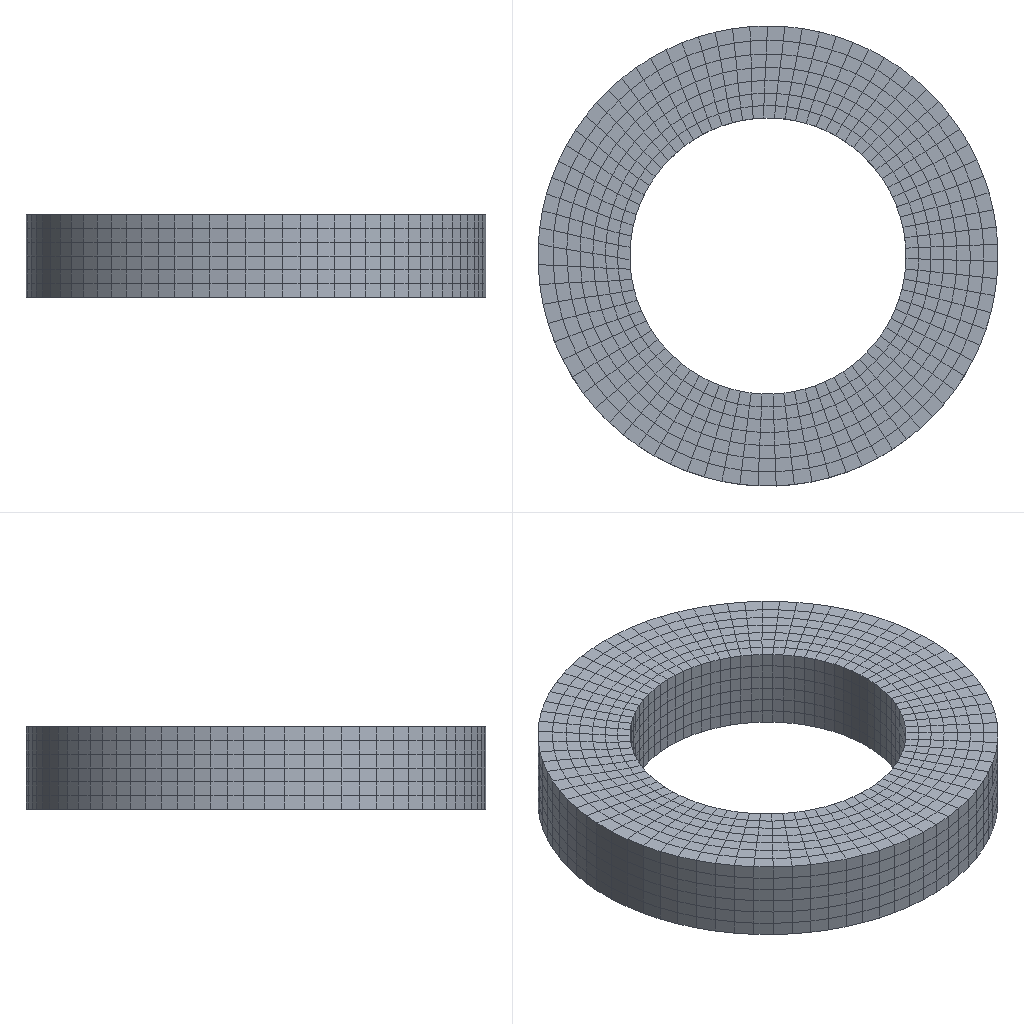Simulation study | abaqus
Set-up summary:
category,name,step,type,value,unit,region
solver,abaqus
solver,version,,,Abaqus/Standard 2020
units,not stated in the deck,,not stated
analysis,deck,,transient,transient
load_step,Step-1,Step-1,transient,nlgeom=True
load_step,Step-2,Step-2,transient,nlgeom=True
contact,interactions,,,general=0 pairs=1 ties=0
load_step,requested,,,2
mesh,nodes,,,5578
mesh,elements,,,4440
element_type,R3D4,,rigid,1038
element_type,C3D8RH,,solid,3402
load,load commands in deck,,count,3
bc,support commands in deck,,count,23
material,PU,,in results
check,setup vs results,,match,"per instance, exact: element labels, types and connectivity; labels of the nodes the elements use; coordinates of those nodes at SINGLE_PRECISION in 2 of 2 instance(s)"
Abaqus input file, long lists of numbers shortened, first 1954 of 6997 lines:
*Heading
** Job name: Job-1 Model name: Job-stress
** Generated by: Abaqus/CAE 2020
*Preprint, echo=NO, model=NO, history=NO, contact=NO
**
** PARTS
**
*Part, name=PART-1
*Node
      1,   21.965,   44.917,           0.
      2,   12.595,   27.228,           0.
** (4535 more lines like these left out)
*Element, type=C3D8RH
   1,  649,  659,  841,  720,    1,   11,  193,   72
   2,  659,  660,  842,  841,   11,   12,  194,  193
** (3400 more lines like these left out)
*Elset, elset=PART-1-1_SHIXINTAI, generate
    1,  3402,     1
** Section: Section-1-PART-1-1_SHIXINTAI
*Solid Section, elset=PART-1-1_SHIXINTAI, material=PU
,
*End Part
**
*Part, name=road
*Node
      1,         200.,           0.,           1.
      2,         200.,        -150.,           1.
** (1038 more lines like these left out)
*Element, type=R3D4
 1,  1,  9, 44,  4
 2,  9, 10, 43, 44
** (1036 more lines like these left out)
*Node
   1041,         100.,         -75.,           0.
*Nset, nset=road-RefPt_, internal
1041,
*Elset, elset=road, generate
    1,  1038,     1
*End Part
**
**
** ASSEMBLY
**
*Assembly, name=Assembly
**
*Instance, name=PART-1-1, part=PART-1
*End Instance
**
*Instance, name=road-1, part=road
         20.,         -51.,         -85.
         20.,         -51.,         -85.,          20., -50.293, -85.707,         180.
*End Instance
**
*Nset, nset=PART-1-1_NEI-RP, instance=PART-1-1
 4537,
*Nset, nset=Set-3417, instance=road-1
 1041,
*Nset, nset=PART-1-1-REFPT_, internal, instance=PART-1-1
 4537,
*Elset, elset=_M18, internal, instance=PART-1-1
 1188,
*Elset, elset=_M19, internal, instance=PART-1-1
 1181,
*Elset, elset=_M20, internal, instance=PART-1-1
 1755,
*Elset, elset=_M21, internal, instance=PART-1-1
 1174,
*Elset, elset=_M22, internal, instance=PART-1-1
 1087,
*Elset, elset=_M23, internal, instance=PART-1-1
 1655,
*Elset, elset=_M24, internal, instance=PART-1-1
 1195,
*Elset, elset=_M25, internal, instance=PART-1-1
 1648,
*Elset, elset=_M26, internal, instance=PART-1-1
 1762,
*Elset, elset=_M27, internal, instance=PART-1-1
 1748,
*Elset, elset=_M28, internal, instance=PART-1-1
 1634,
*Elset, elset=_M29, internal, instance=PART-1-1
 1641,
*Elset, elset=_M30, internal, instance=PART-1-1
 1167,
*Elset, elset=_M31, internal, instance=PART-1-1
 1662,
*Elset, elset=_M32, internal, instance=PART-1-1
 1202,
*Elset, elset=_M33, internal, instance=PART-1-1
 1769,
*Elset, elset=_M34, internal, instance=PART-1-1
 2229,
*Elset, elset=_M35, internal, instance=PART-1-1
 1073,
*Elset, elset=_M36, internal, instance=PART-1-1
 1091,
*Elset, elset=_M37, internal, instance=PART-1-1
 1180,
*Elset, elset=_M38, internal, instance=PART-1-1
 1741,
*Elset, elset=_M39, internal, instance=PART-1-1
 1084,
*Elset, elset=_M40, internal, instance=PART-1-1
 2215,
*Elset, elset=_M41, internal, instance=PART-1-1
 1187,
*Elset, elset=_M42, internal, instance=PART-1-1
 1063,
*Elset, elset=_M43, internal, instance=PART-1-1
 1642,
*Elset, elset=_M44, internal, instance=PART-1-1
 1650,
*Elset, elset=_M45, internal, instance=PART-1-1
 1098,
*Elset, elset=_M46, internal, instance=PART-1-1
 1194,
*Elset, elset=_M47, internal, instance=PART-1-1
 1649,
*Elset, elset=_M48, internal, instance=PART-1-1
 1172,
*Elset, elset=_M49, internal, instance=PART-1-1
 1656,
*Elset, elset=_M50, internal, instance=PART-1-1
 1643,
*Elset, elset=_M51, internal, instance=PART-1-1
 1179,
*Elset, elset=_M52, internal, instance=PART-1-1
 1166,
*Elset, elset=_M53, internal, instance=PART-1-1
 2236,
*Elset, elset=_M54, internal, instance=PART-1-1
 1173,
*Elset, elset=_M55, internal, instance=PART-1-1
 1663,
*Elset, elset=_M56, internal, instance=PART-1-1
 1669,
*Elset, elset=_M57, internal, instance=PART-1-1
 1627,
*Elset, elset=_M58, internal, instance=PART-1-1
 2208,
*Elset, elset=_M59, internal, instance=PART-1-1
 1160,
*Elset, elset=_M60, internal, instance=PART-1-1
 1165,
*Elset, elset=_M61, internal, instance=PART-1-1
 1761,
*Elset, elset=_M62, internal, instance=PART-1-1
 1635,
*Elset, elset=_M63, internal, instance=PART-1-1
 2222,
*Elset, elset=_M64, internal, instance=PART-1-1
 1754,
*Elset, elset=_M65, internal, instance=PART-1-1
 1657,
*Elset, elset=_M66, internal, instance=PART-1-1
 1636,
*Elset, elset=_M67, internal, instance=PART-1-1
 2217,
*Elset, elset=_M68, internal, instance=PART-1-1
 1159,
*Elset, elset=_M69, internal, instance=PART-1-1
 1201,
*Elset, elset=_M70, internal, instance=PART-1-1
 1768,
*Elset, elset=_M71, internal, instance=PART-1-1
 1059,
*Elset, elset=_M72, internal, instance=PART-1-1
 1209,
*Elset, elset=_M73, internal, instance=PART-1-1
 1186,
*Elset, elset=_M74, internal, instance=PART-1-1
 1747,
*Elset, elset=_M75, internal, instance=PART-1-1
 1776,
*Elset, elset=_M76, internal, instance=PART-1-1
 2194,
*Elset, elset=_M77, internal, instance=PART-1-1
 1734,
*Elset, elset=_M78, internal, instance=PART-1-1
 2788,
*Elset, elset=_M79, internal, instance=PART-1-1
 2210,
*Elset, elset=_M80, internal, instance=PART-1-1
 601,
*Elset, elset=_M81, internal, instance=PART-1-1
 611,
*Elset, elset=_M82, internal, instance=PART-1-1
 1629,
*Elset, elset=_M83, internal, instance=PART-1-1
 2201,
*Elset, elset=_M84, internal, instance=PART-1-1
 2230,
*Elset, elset=_M85, internal, instance=PART-1-1
 1670,
*Elset, elset=_M86, internal, instance=PART-1-1
 1628,
*Elset, elset=_M87, internal, instance=PART-1-1
 1753,
*Elset, elset=_M88, internal, instance=PART-1-1
 2223,
*Elset, elset=_M89, internal, instance=PART-1-1
 1746,
*Elset, elset=_M90, internal, instance=PART-1-1
 2209,
*Elset, elset=_M91, internal, instance=PART-1-1
 1193,
*Elset, elset=_M92, internal, instance=PART-1-1
 1739,
*Elset, elset=_M93, internal, instance=PART-1-1
 1153,
*Elset, elset=_M94, internal, instance=PART-1-1
 1740,
*Elset, elset=_M95, internal, instance=PART-1-1
 2216,
*Elset, elset=_M96, internal, instance=PART-1-1
 2224,
*Elset, elset=_M97, internal, instance=PART-1-1
 1676,
*Elset, elset=_M98, internal, instance=PART-1-1
 594,
*Elset, elset=_M99, internal, instance=PART-1-1
 1760,
*Elset, elset=_M100, internal, instance=PART-1-1
 1208,
*Elset, elset=_M101, internal, instance=PART-1-1
 1158,
*Elset, elset=_M102, internal, instance=PART-1-1
 597,
*Elset, elset=_M103, internal, instance=PART-1-1
 1664,
*Elset, elset=_M104, internal, instance=PART-1-1
 2237,
*Elset, elset=_M105, internal, instance=PART-1-1
 1066,
*Elset, elset=_M106, internal, instance=PART-1-1
 1200,
*Elset, elset=_M107, internal, instance=PART-1-1
 1775,
*Elset, elset=_M108, internal, instance=PART-1-1
 1733,
*Elset, elset=_M109, internal, instance=PART-1-1
 1620,
*Elset, elset=_M110, internal, instance=PART-1-1
 1767,
*Elset, elset=_M111, internal, instance=PART-1-1
 1732,
*Elset, elset=_M112, internal, instance=PART-1-1
 2243,
*Elset, elset=_M113, internal, instance=PART-1-1
 1677,
*Elset, elset=_M114, internal, instance=PART-1-1
 1727,
*Elset, elset=_M115, internal, instance=PART-1-1
 1152,
*Elset, elset=_M116, internal, instance=PART-1-1
 1725,
*Elset, elset=_M117, internal, instance=PART-1-1
 604,
*Elset, elset=_M118, internal, instance=PART-1-1
 1726,
*Elset, elset=_M119, internal, instance=PART-1-1
 1621,
*Elset, elset=_M120, internal, instance=PART-1-1
 1749,
*Elset, elset=_M121, internal, instance=PART-1-1
 2203,
*Elset, elset=_M122, internal, instance=PART-1-1
 1207,
*Elset, elset=_M123, internal, instance=PART-1-1
 1182,
*Elset, elset=_M124, internal, instance=PART-1-1
 1720,
*Elset, elset=_M125, internal, instance=PART-1-1
 590,
*Elset, elset=_M126, internal, instance=PART-1-1
 1151,
*Elset, elset=_M127, internal, instance=PART-1-1
 1489,
*Elset, elset=_M128, internal, instance=PART-1-1
 615,
*Elset, elset=_M129, internal, instance=PART-1-1
 1719,
*Elset, elset=_M130, internal, instance=PART-1-1
 2231,
*Elset, elset=_M131, internal, instance=PART-1-1
 1622,
*Elset, elset=_M132, internal, instance=PART-1-1
 1671,
*Elset, elset=_M133, internal, instance=PART-1-1
 1215,
*Elset, elset=_M134, internal, instance=PART-1-1
 2244,
*Elset, elset=_M135, internal, instance=PART-1-1
 2187,
*Elset, elset=_M136, internal, instance=PART-1-1
 2202,
*Elset, elset=_M137, internal, instance=PART-1-1
 1774,
*Elset, elset=_M138, internal, instance=PART-1-1
 1145,
*Elset, elset=_M139, internal, instance=PART-1-1
 1496,
*Elset, elset=_M140, internal, instance=PART-1-1
 1488,
*Elset, elset=_M141, internal, instance=PART-1-1
 1216,
*Elset, elset=_M142, internal, instance=PART-1-1
 608,
*Elset, elset=_M143, internal, instance=PART-1-1
 622,
*Elset, elset=_M144, internal, instance=PART-1-1
 2056,
*Elset, elset=_M145, internal, instance=PART-1-1
 1146,
*Elset, elset=_M146, internal, instance=PART-1-1
 2340,
*Elset, elset=_M147, internal, instance=PART-1-1
 1782,
*Elset, elset=_M148, internal, instance=PART-1-1
 1712,
*Elset, elset=_M149, internal, instance=PART-1-1
 2063,
*Elset, elset=_M150, internal, instance=PART-1-1
 1077,
*Elset, elset=_M151, internal, instance=PART-1-1
 1214,
*Elset, elset=_M152, internal, instance=PART-1-1
 1713,
*Elset, elset=_M153, internal, instance=PART-1-1
 2189,
*Elset, elset=_M154, internal, instance=PART-1-1
 1718,
*Elset, elset=_M155, internal, instance=PART-1-1
 919,
*Elset, elset=_M156, internal, instance=PART-1-1
 2238,
*Elset, elset=_M157, internal, instance=PART-1-1
 1783,
*Elset, elset=_M158, internal, instance=PART-1-1
 2055,
*Elset, elset=_M159, internal, instance=PART-1-1
 2207,
*Elset, elset=_M160, internal, instance=PART-1-1
 2195,
*Elset, elset=_M161, internal, instance=PART-1-1
 1495,
*Elset, elset=_M162, internal, instance=PART-1-1
 1684,
*Elset, elset=_M163, internal, instance=PART-1-1
 2196,
*Elset, elset=_M164, internal, instance=PART-1-1
 1503,
*Elset, elset=_M165, internal, instance=PART-1-1
 1711,
*Elset, elset=_M166, internal, instance=PART-1-1
 1144,
*Elset, elset=_M167, internal, instance=PART-1-1
 1138,
*Elset, elset=_M168, internal, instance=PART-1-1
 2070,
*Elset, elset=_M169, internal, instance=PART-1-1
 2188,
*Elset, elset=_M170, internal, instance=PART-1-1
 1678,
*Elset, elset=_M171, internal, instance=PART-1-1
 2062,
*Elset, elset=_M172, internal, instance=PART-1-1
 1487,
*Elset, elset=_M173, internal, instance=PART-1-1
 2245,
*Elset, elset=_M174, internal, instance=PART-1-1
 2799,
*Elset, elset=_M175, internal, instance=PART-1-1
 1683,
*Elset, elset=_M176, internal, instance=PART-1-1
 1222,
*Elset, elset=_M177, internal, instance=PART-1-1
 1139,
*Elset, elset=_M178, internal, instance=PART-1-1
 1781,
*Elset, elset=_M179, internal, instance=PART-1-1
 1055,
*Elset, elset=_M180, internal, instance=PART-1-1
 1705,
*Elset, elset=_M181, internal, instance=PART-1-1
 629,
*Elset, elset=_M182, internal, instance=PART-1-1
 2250,
*Elset, elset=_M183, internal, instance=PART-1-1
 1223,
*Elset, elset=_M184, internal, instance=PART-1-1
 1706,
*Elset, elset=_M185, internal, instance=PART-1-1
 1790,
*Elset, elset=_M186, internal, instance=PART-1-1
 1789,
*Elset, elset=_M187, internal, instance=PART-1-1
 1137,
*Elset, elset=_M188, internal, instance=PART-1-1
 1052,
*Elset, elset=_M189, internal, instance=PART-1-1
 1502,
*Elset, elset=_M190, internal, instance=PART-1-1
 1704,
*Elset, elset=_M191, internal, instance=PART-1-1
 2251,
*Elset, elset=_M192, internal, instance=PART-1-1
 2312,
*Elset, elset=_M193, internal, instance=PART-1-1
 587,
*Elset, elset=_M194, internal, instance=PART-1-1
 2069,
*Elset, elset=_M195, internal, instance=PART-1-1
 2809,
*Elset, elset=_M196, internal, instance=PART-1-1
 2291,
*Elset, elset=_M197, internal, instance=PART-1-1
 1685,
*Elset, elset=_M198, internal, instance=PART-1-1
 2802,
*Elset, elset=_M199, internal, instance=PART-1-1
 2760,
*Elset, elset=_M200, internal, instance=PART-1-1
 1101,
*Elset, elset=_M201, internal, instance=PART-1-1
 2781,
*Elset, elset=_M202, internal, instance=PART-1-1
 1320,
*Elset, elset=_M203, internal, instance=PART-1-1
 2252,
*Elset, elset=_M204, internal, instance=PART-1-1
 1509,
*Elset, elset=_M205, internal, instance=PART-1-1
 2054,
*Elset, elset=_M206, internal, instance=PART-1-1
 2077,
*Elset, elset=_M207, internal, instance=PART-1-1
 1221,
*Elset, elset=_M208, internal, instance=PART-1-1
 1229,
*Elset, elset=_M209, internal, instance=PART-1-1
 1494,
*Elset, elset=_M210, internal, instance=PART-1-1
 1886,
*Elset, elset=_M211, internal, instance=PART-1-1
 1691,
*Elset, elset=_M212, internal, instance=PART-1-1
 2753,
*Elset, elset=_M213, internal, instance=PART-1-1
 1887,
*Elset, elset=_M214, internal, instance=PART-1-1
 1510,
*Elset, elset=_M215, internal, instance=PART-1-1
 1319,
*Elset, elset=_M216, internal, instance=PART-1-1
 1230,
*Elset, elset=_M217, internal, instance=PART-1-1
 583,
*Elset, elset=_M218, internal, instance=PART-1-1
 947,
*Elset, elset=_M219, internal, instance=PART-1-1
 1796,
*Elset, elset=_M220, internal, instance=PART-1-1
 1788,
*Elset, elset=_M221, internal, instance=PART-1-1
 2061,
*Elset, elset=_M222, internal, instance=PART-1-1
 1797,
*Elset, elset=_M223, internal, instance=PART-1-1
 1074,
*Elset, elset=_M224, internal, instance=PART-1-1
 2813,
*Elset, elset=_M225, internal, instance=PART-1-1
 2309,
*Elset, elset=_M226, internal, instance=PART-1-1
 1501,
*Elset, elset=_M227, internal, instance=PART-1-1
 2076,
*Elset, elset=_M228, internal, instance=PART-1-1
 2774,
*Elset, elset=_M229, internal, instance=PART-1-1
 2638,
*Elset, elset=_M230, internal, instance=PART-1-1
 755,
*Elset, elset=_M231, internal, instance=PART-1-1
 2277,
*Elset, elset=_M232, internal, instance=PART-1-1
 1516,
*Elset, elset=_M233, internal, instance=PART-1-1
 1893,
*Elset, elset=_M234, internal, instance=PART-1-1
 2764,
*Elset, elset=_M235, internal, instance=PART-1-1
 1321,
*Elset, elset=_M236, internal, instance=PART-1-1
 1692,
*Elset, elset=_M237, internal, instance=PART-1-1
 2075,
*Elset, elset=_M238, internal, instance=PART-1-1
 1508,
*Elset, elset=_M239, internal, instance=PART-1-1
 1185,
*Elset, elset=_M240, internal, instance=PART-1-1
 1894,
*Elset, elset=_M241, internal, instance=PART-1-1
 1327,
*Elset, elset=_M242, internal, instance=PART-1-1
 1690,
*Elset, elset=_M243, internal, instance=PART-1-1
 2084,
*Elset, elset=_M244, internal, instance=PART-1-1
 1326,
*Elset, elset=_M245, internal, instance=PART-1-1
 1888,
*Elset, elset=_M246, internal, instance=PART-1-1
 2068,
*Elset, elset=_M247, internal, instance=PART-1-1
 1517,
*Elset, elset=_M248, internal, instance=PART-1-1
 2258,
*Elset, elset=_M249, internal, instance=PART-1-1
 2083,
*Elset, elset=_M250, internal, instance=PART-1-1
 2757,
*Elset, elset=_M251, internal, instance=PART-1-1
 2284,
*Elset, elset=_M252, internal, instance=PART-1-1
 2270,
*Elset, elset=_M253, internal, instance=PART-1-1
 1126,
*Elset, elset=_M254, internal, instance=PART-1-1
 2771,
*Elset, elset=_M255, internal, instance=PART-1-1
 1228,
*Elset, elset=_M256, internal, instance=PART-1-1
 2778,
*Elset, elset=_M257, internal, instance=PART-1-1
 1164,
*Elset, elset=_M258, internal, instance=PART-1-1
 1236,
*Elset, elset=_M259, internal, instance=PART-1-1
 1088,
*Elset, elset=_M260, internal, instance=PART-1-1
 2305,
*Elset, elset=_M261, internal, instance=PART-1-1
 2624,
*Elset, elset=_M262, internal, instance=PART-1-1
 1334,
*Elset, elset=_M263, internal, instance=PART-1-1
 2257,
*Elset, elset=_M264, internal, instance=PART-1-1
 1119,
*Elset, elset=_M265, internal, instance=PART-1-1
 2259,
*Elset, elset=_M266, internal, instance=PART-1-1
 1803,
*Elset, elset=_M267, internal, instance=PART-1-1
 1515,
*Elset, elset=_M268, internal, instance=PART-1-1
 1901,
*Elset, elset=_M269, internal, instance=PART-1-1
 2456,
*Elset, elset=_M270, internal, instance=PART-1-1
 1698,
*Elset, elset=_M271, internal, instance=PART-1-1
 1640,
*Elset, elset=_M272, internal, instance=PART-1-1
 1333,
*Elset, elset=_M273, internal, instance=PART-1-1
 643,
*Elset, elset=_M274, internal, instance=PART-1-1
 569,
*Elset, elset=_M275, internal, instance=PART-1-1
 1237,
*Elset, elset=_M276, internal, instance=PART-1-1
 2057,
*Elset, elset=_M277, internal, instance=PART-1-1
 2326,
*Elset, elset=_M278, internal, instance=PART-1-1
 765,
*Elset, elset=_M279, internal, instance=PART-1-1
 1795,
*Elset, elset=_M280, internal, instance=PART-1-1
 1112,
*Elset, elset=_M281, internal, instance=PART-1-1
 1900,
*Elset, elset=_M282, internal, instance=PART-1-1
 626,
*Elset, elset=_M283, internal, instance=PART-1-1
 1523,
*Elset, elset=_M284, internal, instance=PART-1-1
 2082,
*Elset, elset=_M285, internal, instance=PART-1-1
 1895,
*Elset, elset=_M286, internal, instance=PART-1-1
 1752,
*Elset, elset=_M287, internal, instance=PART-1-1
 2298,
*Elset, elset=_M288, internal, instance=PART-1-1
 1341,
*Elset, elset=_M289, internal, instance=PART-1-1
 2090,
*Elset, elset=_M290, internal, instance=PART-1-1
 636,
*Elset, elset=_M291, internal, instance=PART-1-1
 607,
*Elset, elset=_M292, internal, instance=PART-1-1
 1908,
*Elset, elset=_M293, internal, instance=PART-1-1
 1056,
*Elset, elset=_M294, internal, instance=PART-1-1
 758,
*Elset, elset=_M295, internal, instance=PART-1-1
 2816,
*Elset, elset=_M296, internal, instance=PART-1-1
 1637,
*Elset, elset=_M297, internal, instance=PART-1-1
 2823,
*Elset, elset=_M298, internal, instance=PART-1-1
 1243,
*Elset, elset=_M299, internal, instance=PART-1-1
 1328,
*Elset, elset=_M300, internal, instance=PART-1-1
 1804,
*Elset, elset=_M301, internal, instance=PART-1-1
 2767,
*Elset, elset=_M302, internal, instance=PART-1-1
 1697,
*Elset, elset=_M303, internal, instance=PART-1-1
 2089,
*Elset, elset=_M304, internal, instance=PART-1-1
 1340,
*Elset, elset=_M305, internal, instance=PART-1-1
 1171,
*Elset, elset=_M306, internal, instance=PART-1-1
 2091,
*Elset, elset=_M307, internal, instance=PART-1-1
 1129,
*Elset, elset=_M308, internal, instance=PART-1-1
 2795,
*Elset, elset=_M309, internal, instance=PART-1-1
 580,
*Elset, elset=_M310, internal, instance=PART-1-1
 1522,
*Elset, elset=_M311, internal, instance=PART-1-1
 1335,
*Elset, elset=_M312, internal, instance=PART-1-1
 1524,
*Elset, elset=_M313, internal, instance=PART-1-1
 1907,
*Elset, elset=_M314, internal, instance=PART-1-1
 2265,
*Elset, elset=_M315, internal, instance=PART-1-1
 1235,
*Elset, elset=_M316, internal, instance=PART-1-1
 2652,
*Elset, elset=_M317, internal, instance=PART-1-1
 1699,
*Elset, elset=_M318, internal, instance=PART-1-1
 975,
*Elset, elset=_M319, internal, instance=PART-1-1
 1902,
*Elset, elset=_M320, internal, instance=PART-1-1
 2645,
*Elset, elset=_M321, internal, instance=PART-1-1
 618,
*Elset, elset=_M322, internal, instance=PART-1-1
 1530,
*Elset, elset=_M323, internal, instance=PART-1-1
 1411,
*Elset, elset=_M324, internal, instance=PART-1-1
 1213,
*Elset, elset=_M325, internal, instance=PART-1-1
 2264,
*Elset, elset=_M326, internal, instance=PART-1-1
 642,
*Elset, elset=_M327, internal, instance=PART-1-1
 1802,
*Elset, elset=_M328, internal, instance=PART-1-1
 2329,
*Elset, elset=_M329, internal, instance=PART-1-1
 1490,
*Elset, elset=_M330, internal, instance=PART-1-1
 632,
*Elset, elset=_M331, internal, instance=PART-1-1
 1892,
*Elset, elset=_M332, internal, instance=PART-1-1
 2477,
*Elset, elset=_M333, internal, instance=PART-1-1
 922,
*Elset, elset=_M334, internal, instance=PART-1-1
 1810,
*Elset, elset=_M335, internal, instance=PART-1-1
 958,
*Elset, elset=_M336, internal, instance=PART-1-1
 1348,
*Elset, elset=_M337, internal, instance=PART-1-1
 2266,
*Elset, elset=_M338, internal, instance=PART-1-1
 776,
*Elset, elset=_M339, internal, instance=PART-1-1
 1242,
*Elset, elset=_M340, internal, instance=PART-1-1
 2323,
*Elset, elset=_M341, internal, instance=PART-1-1
 2335,
*Elset, elset=_M342, internal, instance=PART-1-1
 2806,
*Elset, elset=_M343, internal, instance=PART-1-1
 1250,
*Elset, elset=_M344, internal, instance=PART-1-1
 1909,
*Elset, elset=_M345, internal, instance=PART-1-1
 1889,
*Elset, elset=_M346, internal, instance=PART-1-1
 1915,
*Elset, elset=_M347, internal, instance=PART-1-1
 2470,
*Elset, elset=_M348, internal, instance=PART-1-1
 1342,
*Elset, elset=_M349, internal, instance=PART-1-1
 951,
*Elset, elset=_M350, internal, instance=PART-1-1
 2097,
*Elset, elset=_M351, internal, instance=PART-1-1
 598,
*Elset, elset=_M352, internal, instance=PART-1-1
 2281,
*Elset, elset=_M353, internal, instance=PART-1-1
 2344,
*Elset, elset=_M354, internal, instance=PART-1-1
 1102,
*Elset, elset=_M355, internal, instance=PART-1-1
 1244,
*Elset, elset=_M356, internal, instance=PART-1-1
 1097,
*Elset, elset=_M357, internal, instance=PART-1-1
 1809,
*Elset, elset=_M358, internal, instance=PART-1-1
 619,
*Elset, elset=_M359, internal, instance=PART-1-1
 579,
*Elset, elset=_M360, internal, instance=PART-1-1
 1322,
*Elset, elset=_M361, internal, instance=PART-1-1
 1110,
*Elset, elset=_M362, internal, instance=PART-1-1
 1412,
*Elset, elset=_M363, internal, instance=PART-1-1
 1531,
*Elset, elset=_M364, internal, instance=PART-1-1
 1410,
*Elset, elset=_M365, internal, instance=PART-1-1
 2827,
*Elset, elset=_M366, internal, instance=PART-1-1
 592,
*Elset, elset=_M367, internal, instance=PART-1-1
 1529,
*Elset, elset=_M368, internal, instance=PART-1-1
 2820,
*Elset, elset=_M369, internal, instance=PART-1-1
 2634,
*Elset, elset=_M370, internal, instance=PART-1-1
 2186,
*Elset, elset=_M371, internal, instance=PART-1-1
 1537,
*Elset, elset=_M372, internal, instance=PART-1-1
 1978,
*Elset, elset=_M373, internal, instance=PART-1-1
 1977,
*Elset, elset=_M374, internal, instance=PART-1-1
 1916,
*Elset, elset=_M375, internal, instance=PART-1-1
 2096,
*Elset, elset=_M376, internal, instance=PART-1-1
 2204,
*Elset, elset=_M377, internal, instance=PART-1-1
 1083,
*Elset, elset=_M378, internal, instance=PART-1-1
 2358,
*Elset, elset=_M379, internal, instance=PART-1-1
 1061,
*Elset, elset=_M380, internal, instance=PART-1-1
 1178,
*Elset, elset=_M381, internal, instance=PART-1-1
 2659,
*Elset, elset=_M382, internal, instance=PART-1-1
 769,
*Elset, elset=_M383, internal, instance=PART-1-1
 1418,
*Elset, elset=_M384, internal, instance=PART-1-1
 1355,
*Elset, elset=_M385, internal, instance=PART-1-1
 2098,
*Elset, elset=_M386, internal, instance=PART-1-1
 1672,
*Elset, elset=_M387, internal, instance=PART-1-1
 640,
*Elset, elset=_M388, internal, instance=PART-1-1
 2239,
*Elset, elset=_M389, internal, instance=PART-1-1
 1914,
*Elset, elset=_M390, internal, instance=PART-1-1
 1922,
*Elset, elset=_M391, internal, instance=PART-1-1
 2830,
*Elset, elset=_M392, internal, instance=PART-1-1
 1349,
*Elset, elset=_M393, internal, instance=PART-1-1
 944,
*Elset, elset=_M394, internal, instance=PART-1-1
 2459,
*Elset, elset=_M395, internal, instance=PART-1-1
 2306,
*Elset, elset=_M396, internal, instance=PART-1-1
 1885,
*Elset, elset=_M397, internal, instance=PART-1-1
 657,
*Elset, elset=_M398, internal, instance=PART-1-1
 1054,
*Elset, elset=_M399, internal, instance=PART-1-1
 1175,
*Elset, elset=_M400, internal, instance=PART-1-1
 2351,
*Elset, elset=_M401, internal, instance=PART-1-1
 2104,
*Elset, elset=_M402, internal, instance=PART-1-1
 2347,
*Elset, elset=_M403, internal, instance=PART-1-1
 1817,
*Elset, elset=_M404, internal, instance=PART-1-1
 1738,
*Elset, elset=_M405, internal, instance=PART-1-1
 2302,
*Elset, elset=_M406, internal, instance=PART-1-1
 1060,
*Elset, elset=_M407, internal, instance=PART-1-1
 650,
*Elset, elset=_M408, internal, instance=PART-1-1
 2455,
*Elset, elset=_M409, internal, instance=PART-1-1
 1724,
*Elset, elset=_M410, internal, instance=PART-1-1
 940,
*Elset, elset=_M411, internal, instance=PART-1-1
 2798,
*Elset, elset=_M412, internal, instance=PART-1-1
 1249,
*Elset, elset=_M413, internal, instance=PART-1-1
 2316,
*Elset, elset=_M414, internal, instance=PART-1-1
 2491,
*Elset, elset=_M415, internal, instance=PART-1-1
 1816,
*Elset, elset=_M416, internal, instance=PART-1-1
 2253,
*Elset, elset=_M417, internal, instance=PART-1-1
 1979,
*Elset, elset=_M418, internal, instance=PART-1-1
 1347,
*Elset, elset=_M419, internal, instance=PART-1-1
 1154,
*Elset, elset=_M420, internal, instance=PART-1-1
 2333,
*Elset, elset=_M421, internal, instance=PART-1-1
 613,
*Elset, elset=_M422, internal, instance=PART-1-1
 1257,
*Elset, elset=_M423, internal, instance=PART-1-1
 1811,
*Elset, elset=_M424, internal, instance=PART-1-1
 667,
*Elset, elset=_M425, internal, instance=PART-1-1
 1256,
*Elset, elset=_M426, internal, instance=PART-1-1
 1133,
*Elset, elset=_M427, internal, instance=PART-1-1
 2484,
*Elset, elset=_M428, internal, instance=PART-1-1
 762,
*Elset, elset=_M429, internal, instance=PART-1-1
 2357,
*Elset, elset=_M430, internal, instance=PART-1-1
 1544,
*Elset, elset=_M431, internal, instance=PART-1-1
 842,
*Elset, elset=_M432, internal, instance=PART-1-1
 1923,
*Elset, elset=_M433, internal, instance=PART-1-1
 2620,
*Elset, elset=_M434, internal, instance=PART-1-1
 1251,
*Elset, elset=_M435, internal, instance=PART-1-1
 761,
*Elset, elset=_M436, internal, instance=PART-1-1
 790,
*Elset, elset=_M437, internal, instance=PART-1-1
 653,
*Elset, elset=_M438, internal, instance=PART-1-1
 2636,
*Elset, elset=_M439, internal, instance=PART-1-1
 633,
*Elset, elset=_M440, internal, instance=PART-1-1
 1536,
*Elset, elset=_M441, internal, instance=PART-1-1
 681,
*Elset, elset=_M442, internal, instance=PART-1-1
 2463,
*Elset, elset=_M443, internal, instance=PART-1-1
 1419,
*Elset, elset=_M444, internal, instance=PART-1-1
 1538,
*Elset, elset=_M445, internal, instance=PART-1-1
 1985,
*Elset, elset=_M446, internal, instance=PART-1-1
 678,
*Elset, elset=_M447, internal, instance=PART-1-1
 2803,
*Elset, elset=_M448, internal, instance=PART-1-1
 1220,
*Elset, elset=_M449, internal, instance=PART-1-1
 1143,
*Elset, elset=_M450, internal, instance=PART-1-1
 649,
*Elset, elset=_M451, internal, instance=PART-1-1
 1362,
*Elset, elset=_M452, internal, instance=PART-1-1
 1651,
*Elset, elset=_M453, internal, instance=PART-1-1
 1742,
*Elset, elset=_M454, internal, instance=PART-1-1
 1824,
*Elset, elset=_M455, internal, instance=PART-1-1
 965,
*Elset, elset=_M456, internal, instance=PART-1-1
 2498,
*Elset, elset=_M457, internal, instance=PART-1-1
 1095,
*Elset, elset=_M458, internal, instance=PART-1-1
 2396,
*Elset, elset=_M459, internal, instance=PART-1-1
 576,
*Elset, elset=_M460, internal, instance=PART-1-1
 660,
*Elset, elset=_M461, internal, instance=PART-1-1
 1105,
*Elset, elset=_M462, internal, instance=PART-1-1
 1497,
*Elset, elset=_M463, internal, instance=PART-1-1
 1766,
*Elset, elset=_M464, internal, instance=PART-1-1
 2334,
*Elset, elset=_M465, internal, instance=PART-1-1
 2221,
*Elset, elset=_M466, internal, instance=PART-1-1
 1654,
*Elset, elset=_M467, internal, instance=PART-1-1
 2105,
*Elset, elset=_M468, internal, instance=PART-1-1
 1425,
*Elset, elset=_M469, internal, instance=PART-1-1
 1703,
*Elset, elset=_M470, internal, instance=PART-1-1
 942,
*Elset, elset=_M471, internal, instance=PART-1-1
 1090,
*Elset, elset=_M472, internal, instance=PART-1-1
 1823,
*Elset, elset=_M473, internal, instance=PART-1-1
 1199,
*Elset, elset=_M474, internal, instance=PART-1-1
 933,
*Elset, elset=_M475, internal, instance=PART-1-1
 1116,
*Elset, elset=_M476, internal, instance=PART-1-1
 1264,
*Elset, elset=_M477, internal, instance=PART-1-1
 1929,
*Elset, elset=_M478, internal, instance=PART-1-1
 664,
*Elset, elset=_M479, internal, instance=PART-1-1
 584,
*Elset, elset=_M480, internal, instance=PART-1-1
 1203,
*Elset, elset=_M481, internal, instance=PART-1-1
 2111,
*Elset, elset=_M482, internal, instance=PART-1-1
 620,
*Elset, elset=_M483, internal, instance=PART-1-1
 2103,
*Elset, elset=_M484, internal, instance=PART-1-1
 2319,
*Elset, elset=_M485, internal, instance=PART-1-1
 1356,
*Elset, elset=_M486, internal, instance=PART-1-1
 2361,
*Elset, elset=_M487, internal, instance=PART-1-1
 1417,
*Elset, elset=_M488, internal, instance=PART-1-1
 1543,
*Elset, elset=_M489, internal, instance=PART-1-1
 2053,
*Elset, elset=_M490, internal, instance=PART-1-1
 2382,
*Elset, elset=_M491, internal, instance=PART-1-1
 1551,
*Elset, elset=_M492, internal, instance=PART-1-1
 1325,
*Elset, elset=_M493, internal, instance=PART-1-1
 853,
*Elset, elset=_M494, internal, instance=PART-1-1
 1984,
*Elset, elset=_M495, internal, instance=PART-1-1
 2666,
*Elset, elset=_M496, internal, instance=PART-1-1
 1686,
*Elset, elset=_M497, internal, instance=PART-1-1
 1714,
*Elset, elset=_M498, internal, instance=PART-1-1
 2543,
*Elset, elset=_M499, internal, instance=PART-1-1
 1258,
*Elset, elset=_M500, internal, instance=PART-1-1
 1921,
*Elset, elset=_M501, internal, instance=PART-1-1
 1675,
*Elset, elset=_M502, internal, instance=PART-1-1
 1773,
*Elset, elset=_M503, internal, instance=PART-1-1
 1992,
*Elset, elset=_M504, internal, instance=PART-1-1
 671,
*Elset, elset=_M505, internal, instance=PART-1-1
 1075,
*Elset, elset=_M506, internal, instance=PART-1-1
 1432,
*Elset, elset=_M507, internal, instance=PART-1-1
 1263,
*Elset, elset=_M508, internal, instance=PART-1-1
 1136,
*Elset, elset=_M509, internal, instance=PART-1-1
 928,
*Elset, elset=_M510, internal, instance=PART-1-1
 1831,
*Elset, elset=_M511, internal, instance=PART-1-1
 2804,
*Elset, elset=_M512, internal, instance=PART-1-1
 1271,
*Elset, elset=_M513, internal, instance=PART-1-1
 2641,
*Elset, elset=_M514, internal, instance=PART-1-1
 1426,
*Elset, elset=_M515, internal, instance=PART-1-1
 783,
*Elset, elset=_M516, internal, instance=PART-1-1
 1936,
*Elset, elset=_M517, internal, instance=PART-1-1
 2232,
*Elset, elset=_M518, internal, instance=PART-1-1
 1511,
*Elset, elset=_M519, internal, instance=PART-1-1
 2790,
*Elset, elset=_M520, internal, instance=PART-1-1
 2280,
*Elset, elset=_M521, internal, instance=PART-1-1
 2805,
*Elset, elset=_M522, internal, instance=PART-1-1
 1131,
*Elset, elset=_M523, internal, instance=PART-1-1
 1369,
*Elset, elset=_M524, internal, instance=PART-1-1
 2676,
*Elset, elset=_M525, internal, instance=PART-1-1
 2754,
*Elset, elset=_M526, internal, instance=PART-1-1
 2110,
*Elset, elset=_M527, internal, instance=PART-1-1
 2348,
*Elset, elset=_M528, internal, instance=PART-1-1
 2064,
*Elset, elset=_M529, internal, instance=PART-1-1
 628,
*Elset, elset=_M530, internal, instance=PART-1-1
 1794,
*Elset, elset=_M531, internal, instance=PART-1-1
 1930,
*Elset, elset=_M532, internal, instance=PART-1-1
 923,
*Elset, elset=_M533, internal, instance=PART-1-1
 1096,
*Elset, elset=_M534, internal, instance=PART-1-1
 982,
*Elset, elset=_M535, internal, instance=PART-1-1
 1986,
*Elset, elset=_M536, internal, instance=PART-1-1
 1818,
*Elset, elset=_M537, internal, instance=PART-1-1
 2825,
*Elset, elset=_M538, internal, instance=PART-1-1
 961,
*Elset, elset=_M539, internal, instance=PART-1-1
 1076,
*Elset, elset=_M540, internal, instance=PART-1-1
 2060,
*Elset, elset=_M541, internal, instance=PART-1-1
 1647,
*Elset, elset=_M542, internal, instance=PART-1-1
 1354,
*Elset, elset=_M543, internal, instance=PART-1-1
 2078,
*Elset, elset=_M544, internal, instance=PART-1-1
 786,
*Elset, elset=_M545, internal, instance=PART-1-1
 1439,
*Elset, elset=_M546, internal, instance=PART-1-1
 1999,
*Elset, elset=_M547, internal, instance=PART-1-1
 1363,
*Elset, elset=_M548, internal, instance=PART-1-1
 2321,
*Elset, elset=_M549, internal, instance=PART-1-1
 2118,
*Elset, elset=_M550, internal, instance=PART-1-1
 1227,
*Elset, elset=_M551, internal, instance=PART-1-1
 1545,
*Elset, elset=_M552, internal, instance=PART-1-1
 972,
*Elset, elset=_M553, internal, instance=PART-1-1
 2112,
*Elset, elset=_M554, internal, instance=PART-1-1
 1111,
*Elset, elset=_M555, internal, instance=PART-1-1
 937,
*Elset, elset=_M556, internal, instance=PART-1-1
 2777,
*Elset, elset=_M557, internal, instance=PART-1-1
 2690,
*Elset, elset=_M558, internal, instance=PART-1-1
 1550,
*Elset, elset=_M559, internal, instance=PART-1-1
 1896,
*Elset, elset=_M560, internal, instance=PART-1-1
 1500,
*Elset, elset=_M561, internal, instance=PART-1-1
 1558,
*Elset, elset=_M562, internal, instance=PART-1-1
 793,
*Elset, elset=_M563, internal, instance=PART-1-1
 2006,
*Elset, elset=_M564, internal, instance=PART-1-1
 1756,
*Elset, elset=_M565, internal, instance=PART-1-1
 1830,
*Elset, elset=_M566, internal, instance=PART-1-1
 2673,
*Elset, elset=_M567, internal, instance=PART-1-1
 1318,
*Elset, elset=_M568, internal, instance=PART-1-1
 1825,
*Elset, elset=_M569, internal, instance=PART-1-1
 2662,
*Elset, elset=_M570, internal, instance=PART-1-1
 1361,
*Elset, elset=_M571, internal, instance=PART-1-1
 1943,
*Elset, elset=_M572, internal, instance=PART-1-1
 1343,
*Elset, elset=_M573, internal, instance=PART-1-1
 1928,
*Elset, elset=_M574, internal, instance=PART-1-1
 979,
*Elset, elset=_M575, internal, instance=PART-1-1
 1993,
*Elset, elset=_M576, internal, instance=PART-1-1
 2354,
*Elset, elset=_M577, internal, instance=PART-1-1
 1552,
*Elset, elset=_M578, internal, instance=PART-1-1
 2370,
*Elset, elset=_M579, internal, instance=PART-1-1
 2683,
*Elset, elset=_M580, internal, instance=PART-1-1
 1278,
*Elset, elset=_M581, internal, instance=PART-1-1
 1206,
*Elset, elset=_M582, internal, instance=PART-1-1
 2343,
*Elset, elset=_M583, internal, instance=PART-1-1
 1122,
*Elset, elset=_M584, internal, instance=PART-1-1
 1413,
*Elset, elset=_M585, internal, instance=PART-1-1
 1332,
*Elset, elset=_M586, internal, instance=PART-1-1
 1759,
*Elset, elset=_M587, internal, instance=PART-1-1
 2117,
*Elset, elset=_M588, internal, instance=PART-1-1
 2512,
*Elset, elset=_M589, internal, instance=PART-1-1
 2000,
*Elset, elset=_M590, internal, instance=PART-1-1
 1433,
*Elset, elset=_M591, internal, instance=PART-1-1
 1838,
*Elset, elset=_M592, internal, instance=PART-1-1
 1376,
*Elset, elset=_M593, internal, instance=PART-1-1
 1424,
*Elset, elset=_M594, internal, instance=PART-1-1
 572,
*Elset, elset=_M595, internal, instance=PART-1-1
 2307,
*Elset, elset=_M596, internal, instance=PART-1-1
 656,
*Elset, elset=_M597, internal, instance=PART-1-1
 2067,
*Elset, elset=_M598, internal, instance=PART-1-1
 1707,
*Elset, elset=_M599, internal, instance=PART-1-1
 2776,
*Elset, elset=_M600, internal, instance=PART-1-1
 2403,
*Elset, elset=_M601, internal, instance=PART-1-1
 2342,
*Elset, elset=_M602, internal, instance=PART-1-1
 2125,
*Elset, elset=_M603, internal, instance=PART-1-1
 2575,
*Elset, elset=_M604, internal, instance=PART-1-1
 1493,
*Elset, elset=_M605, internal, instance=PART-1-1
 1446,
*Elset, elset=_M606, internal, instance=PART-1-1
 1837,
*Elset, elset=_M607, internal, instance=PART-1-1
 1370,
*Elset, elset=_M608, internal, instance=PART-1-1
 1234,
*Elset, elset=_M609, internal, instance=PART-1-1
 2294,
*Elset, elset=_M610, internal, instance=PART-1-1
 646,
*Elset, elset=_M611, internal, instance=PART-1-1
 1081,
*Elset, elset=_M612, internal, instance=PART-1-1
 2782,
*Elset, elset=_M613, internal, instance=PART-1-1
 1265,
*Elset, elset=_M614, internal, instance=PART-1-1
 1937,
*Elset, elset=_M615, internal, instance=PART-1-1
 702,
*Elset, elset=_M616, internal, instance=PART-1-1
 1801,
*Elset, elset=_M617, internal, instance=PART-1-1
 1693,
*Elset, elset=_M618, internal, instance=PART-1-1
 1080,
*Elset, elset=_M619, internal, instance=PART-1-1
 2487,
*Elset, elset=_M620, internal, instance=PART-1-1
 2649,
*Elset, elset=_M621, internal, instance=PART-1-1
 1626,
*Elset, elset=_M622, internal, instance=PART-1-1
 2295,
*Elset, elset=_M623, internal, instance=PART-1-1
 2273,
*Elset, elset=_M624, internal, instance=PART-1-1
 1168,
*Elset, elset=_M625, internal, instance=PART-1-1
 1745,
*Elset, elset=_M626, internal, instance=PART-1-1
 845,
*Elset, elset=_M627, internal, instance=PART-1-1
 641,
*Elset, elset=_M628, internal, instance=PART-1-1
 2697,
*Elset, elset=_M629, internal, instance=PART-1-1
 1557,
*Elset, elset=_M630, internal, instance=PART-1-1
 2494,
*Elset, elset=_M631, internal, instance=PART-1-1
 874,
*Elset, elset=_M632, internal, instance=PART-1-1
 2225,
*Elset, elset=_M633, internal, instance=PART-1-1
 1270,
*Elset, elset=_M634, internal, instance=PART-1-1
 849,
*Elset, elset=_M635, internal, instance=PART-1-1
 593,
*Elset, elset=_M636, internal, instance=PART-1-1
 846,
*Elset, elset=_M637, internal, instance=PART-1-1
 571,
*Elset, elset=_M638, internal, instance=PART-1-1
 1845,
*Elset, elset=_M639, internal, instance=PART-1-1
 804,
*Elset, elset=_M640, internal, instance=PART-1-1
 1565,
*Elset, elset=_M641, internal, instance=PART-1-1
 1980,
*Elset, elset=_M642, internal, instance=PART-1-1
 2007,
*Elset, elset=_M643, internal, instance=PART-1-1
 1431,
*Elset, elset=_M644, internal, instance=PART-1-1
 962,
*Elset, elset=_M645, internal, instance=PART-1-1
 1053,
*Elset, elset=_M646, internal, instance=PART-1-1
 1440,
*Elset, elset=_M647, internal, instance=PART-1-1
 2088,
*Elset, elset=_M648, internal, instance=PART-1-1
 751,
*Elset, elset=_M649, internal, instance=PART-1-1
 1991,
*Elset, elset=_M650, internal, instance=PART-1-1
 2242,
*Elset, elset=_M651, internal, instance=PART-1-1
 772,
*Elset, elset=_M652, internal, instance=PART-1-1
 1935,
*Elset, elset=_M653, internal, instance=PART-1-1
 2628,
*Elset, elset=_M654, internal, instance=PART-1-1
 2132,
*Elset, elset=_M655, internal, instance=PART-1-1
 1003,
*Elset, elset=_M656, internal, instance=PART-1-1
 2013,
*Elset, elset=_M657, internal, instance=PART-1-1
 2761,
*Elset, elset=_M658, internal, instance=PART-1-1
 1285,
*Elset, elset=_M659, internal, instance=PART-1-1
 674,
*Elset, elset=_M660, internal, instance=PART-1-1
 2791,
*Elset, elset=_M661, internal, instance=PART-1-1
 1784,
*Elset, elset=_M662, internal, instance=PART-1-1
 2462,
*Elset, elset=_M663, internal, instance=PART-1-1
 1383,
*Elset, elset=_M664, internal, instance=PART-1-1
 1950,
*Elset, elset=_M665, internal, instance=PART-1-1
 1140,
*Elset, elset=_M666, internal, instance=PART-1-1
 2501,
*Elset, elset=_M667, internal, instance=PART-1-1
 1453,
*Elset, elset=_M668, internal, instance=PART-1-1
 1082,
*Elset, elset=_M669, internal, instance=PART-1-1
 1780,
*Elset, elset=_M670, internal, instance=PART-1-1
 1787,
*Elset, elset=_M671, internal, instance=PART-1-1
 800,
*Elset, elset=_M672, internal, instance=PART-1-1
 599,
*Elset, elset=_M673, internal, instance=PART-1-1
 936,
*Elset, elset=_M674, internal, instance=PART-1-1
 577,
*Elset, elset=_M675, internal, instance=PART-1-1
 1336,
*Elset, elset=_M676, internal, instance=PART-1-1
 668,
*Elset, elset=_M677, internal, instance=PART-1-1
 949,
*Elset, elset=_M678, internal, instance=PART-1-1
 2364,
*Elset, elset=_M679, internal, instance=PART-1-1
 1118,
*Elset, elset=_M680, internal, instance=PART-1-1
 1368,
*Elset, elset=_M681, internal, instance=PART-1-1
 2124,
*Elset, elset=_M682, internal, instance=PART-1-1
 811,
*Elset, elset=_M683, internal, instance=PART-1-1
 2119,
*Elset, elset=_M684, internal, instance=PART-1-1
 1844,
*Elset, elset=_M685, internal, instance=PART-1-1
 1644,
*Elset, elset=_M686, internal, instance=PART-1-1
 2627,
*Elset, elset=_M687, internal, instance=PART-1-1
 2817,
*Elset, elset=_M688, internal, instance=PART-1-1
 1899,
*Elset, elset=_M689, internal, instance=PART-1-1
 1852,
*Elset, elset=_M690, internal, instance=PART-1-1
 2267,
*Elset, elset=_M691, internal, instance=PART-1-1
 661,
*Elset, elset=_M692, internal, instance=PART-1-1
 1521,
*Elset, elset=_M693, internal, instance=PART-1-1
 1832,
*Elset, elset=_M694, internal, instance=PART-1-1
 1710,
*Elset, elset=_M695, internal, instance=PART-1-1
 2550,
*Elset, elset=_M696, internal, instance=PART-1-1
 860,
*Elset, elset=_M697, internal, instance=PART-1-1
 1070,
*Elset, elset=_M698, internal, instance=PART-1-1
 2756,
*Elset, elset=_M699, internal, instance=PART-1-1
 1390,
*Elset, elset=_M700, internal, instance=PART-1-1
 1447,
*Elset, elset=_M701, internal, instance=PART-1-1
 2020,
*Elset, elset=_M702, internal, instance=PART-1-1
 2377,
*Elset, elset=_M703, internal, instance=PART-1-1
 921,
*Elset, elset=_M704, internal, instance=PART-1-1
 685,
*Elset, elset=_M705, internal, instance=PART-1-1
 639,
*Elset, elset=_M706, internal, instance=PART-1-1
 1125,
*Elset, elset=_M707, internal, instance=PART-1-1
 1486,
*Elset, elset=_M708, internal, instance=PART-1-1
 2131,
*Elset, elset=_M709, internal, instance=PART-1-1
 2431,
*Elset, elset=_M710, internal, instance=PART-1-1
 2139,
*Elset, elset=_M711, internal, instance=PART-1-1
 818,
*Elset, elset=_M712, internal, instance=PART-1-1
 2755,
*Elset, elset=_M713, internal, instance=PART-1-1
 2337,
*Elset, elset=_M714, internal, instance=PART-1-1
 2327,
*Elset, elset=_M715, internal, instance=PART-1-1
 1957,
*Elset, elset=_M716, internal, instance=PART-1-1
 1668,
*Elset, elset=_M717, internal, instance=PART-1-1
 2554,
*Elset, elset=_M718, internal, instance=PART-1-1
 986,
*Elset, elset=_M719, internal, instance=PART-1-1
 1292,
*Elset, elset=_M720, internal, instance=PART-1-1
 2775,
*Elset, elset=_M721, internal, instance=PART-1-1
 2547,
*Elset, elset=_M722, internal, instance=PART-1-1
 1572,
*Elset, elset=_M723, internal, instance=PART-1-1
 2476,
*Elset, elset=_M724, internal, instance=PART-1-1
 682,
*Elset, elset=_M725, internal, instance=PART-1-1
 2386,
*Elset, elset=_M726, internal, instance=PART-1-1
 797,
*Elset, elset=_M727, internal, instance=PART-1-1
 1067,
*Elset, elset=_M728, internal, instance=PART-1-1
 2308,
*Elset, elset=_M729, internal, instance=PART-1-1
 1147,
*Elset, elset=_M730, internal, instance=PART-1-1
 2368,
*Elset, elset=_M731, internal, instance=PART-1-1
 1350,
*Elset, elset=_M732, internal, instance=PART-1-1
 1277,
*Elset, elset=_M733, internal, instance=PART-1-1
 832,
*Elset, elset=_M734, internal, instance=PART-1-1
 1109,
*Elset, elset=_M735, internal, instance=PART-1-1
 716,
*Elset, elset=_M736, internal, instance=PART-1-1
 968,
*Elset, elset=_M737, internal, instance=PART-1-1
 1579,
*Elset, elset=_M738, internal, instance=PART-1-1
 2146,
*Elset, elset=_M739, internal, instance=PART-1-1
 1559,
*Elset, elset=_M740, internal, instance=PART-1-1
 2762,
*Elset, elset=_M741, internal, instance=PART-1-1
 647,
*Elset, elset=_M742, internal, instance=PART-1-1
 1104,
*Elset, elset=_M743, internal, instance=PART-1-1
 1564,
*Elset, elset=_M744, internal, instance=PART-1-1
 2833,
*Elset, elset=_M745, internal, instance=PART-1-1
 2355,
*Elset, elset=_M746, internal, instance=PART-1-1
 2393,
*Elset, elset=_M747, internal, instance=PART-1-1
 929,
*Elset, elset=_M748, internal, instance=PART-1-1
 926,
*Elset, elset=_M749, internal, instance=PART-1-1
 1377,
*Elset, elset=_M750, internal, instance=PART-1-1
 692,
*Elset, elset=_M751, internal, instance=PART-1-1
 2014,
*Elset, elset=_M752, internal, instance=PART-1-1
 1397,
*Elset, elset=_M753, internal, instance=PART-1-1
 1851,
*Elset, elset=_M754, internal, instance=PART-1-1
 648,
*Elset, elset=_M755, internal, instance=PART-1-1
 1272,
*Elset, elset=_M756, internal, instance=PART-1-1
 1507,
*Elset, elset=_M757, internal, instance=PART-1-1
 2211,
*Elset, elset=_M758, internal, instance=PART-1-1
 1514,
*Elset, elset=_M759, internal, instance=PART-1-1
 1658,
*Elset, elset=_M760, internal, instance=PART-1-1
 1998,
*Elset, elset=_M761, internal, instance=PART-1-1
 635,
*Elset, elset=_M762, internal, instance=PART-1-1
 1284,
*Elset, elset=_M763, internal, instance=PART-1-1
 1903,
*Elset, elset=_M764, internal, instance=PART-1-1
 2796,
*Elset, elset=_M765, internal, instance=PART-1-1
 1460,
*Elset, elset=_M766, internal, instance=PART-1-1
 1586,
*Elset, elset=_M767, internal, instance=PART-1-1
 2313,
*Elset, elset=_M768, internal, instance=PART-1-1
 780,
*Elset, elset=_M769, internal, instance=PART-1-1
 1454,
*Elset, elset=_M770, internal, instance=PART-1-1
 1210,
*Elset, elset=_M771, internal, instance=PART-1-1
 2768,
*Elset, elset=_M772, internal, instance=PART-1-1
 2669,
*Elset, elset=_M773, internal, instance=PART-1-1
 2027,
*Elset, elset=_M774, internal, instance=PART-1-1
 2400,
*Elset, elset=_M775, internal, instance=PART-1-1
 2481,
*Elset, elset=_M776, internal, instance=PART-1-1
 2005,
*Elset, elset=_M777, internal, instance=PART-1-1
 2519,
*Elset, elset=_M778, internal, instance=PART-1-1
 1958,
*Elset, elset=_M779, internal, instance=PART-1-1
 1299,
*Elset, elset=_M780, internal, instance=PART-1-1
 2153,
*Elset, elset=_M781, internal, instance=PART-1-1
 2126,
*Elset, elset=_M782, internal, instance=PART-1-1
 2812,
*Elset, elset=_M783, internal, instance=PART-1-1
 2468,
*Elset, elset=_M784, internal, instance=PART-1-1
 1438,
*Elset, elset=_M785, internal, instance=PART-1-1
 1404,
*Elset, elset=_M786, internal, instance=PART-1-1
 2095,
*Elset, elset=_M787, internal, instance=PART-1-1
 2365,
*Elset, elset=_M788, internal, instance=PART-1-1
 807,
*Elset, elset=_M789, internal, instance=PART-1-1
 1839,
*Elset, elset=_M790, internal, instance=PART-1-1
 950,
*Elset, elset=_M791, internal, instance=PART-1-1
 709,
*Elset, elset=_M792, internal, instance=PART-1-1
 1866,
*Elset, elset=_M793, internal, instance=PART-1-1
 1944,
*Elset, elset=_M794, internal, instance=PART-1-1
 1630,
*Elset, elset=_M795, internal, instance=PART-1-1
 699,
*Elset, elset=_M796, internal, instance=PART-1-1
 1964,
*Elset, elset=_M797, internal, instance=PART-1-1
 767,
*Elset, elset=_M798, internal, instance=PART-1-1
 1942,
*Elset, elset=_M799, internal, instance=PART-1-1
 1859,
*Elset, elset=_M800, internal, instance=PART-1-1
 1467,
*Elset, elset=_M801, internal, instance=PART-1-1
 1375,
*Elset, elset=_M802, internal, instance=PART-1-1
 1364,
*Elset, elset=_M803, internal, instance=PART-1-1
 870,
*Elset, elset=_M804, internal, instance=PART-1-1
 654,
*Elset, elset=_M805, internal, instance=PART-1-1
 2832,
*Elset, elset=_M806, internal, instance=PART-1-1
 1917,
*Elset, elset=_M807, internal, instance=PART-1-1
 1682,
*Elset, elset=_M808, internal, instance=PART-1-1
 2508,
*Elset, elset=_M809, internal, instance=PART-1-1
 2299,
*Elset, elset=_M810, internal, instance=PART-1-1
 2379,
*Elset, elset=_M811, internal, instance=PART-1-1
 1062,
*Elset, elset=_M812, internal, instance=PART-1-1
 2314,
*Elset, elset=_M813, internal, instance=PART-1-1
 1024,
*Elset, elset=_M814, internal, instance=PART-1-1
 1391,
*Elset, elset=_M815, internal, instance=PART-1-1
 1461,
*Elset, elset=_M816, internal, instance=PART-1-1
 1777,
*Elset, elset=_M817, internal, instance=PART-1-1
 2810,
*Elset, elset=_M818, internal, instance=PART-1-1
 1468,
*Elset, elset=_M819, internal, instance=PART-1-1
 1045,
*Elset, elset=_M820, internal, instance=PART-1-1
 2246,
*Elset, elset=_M821, internal, instance=PART-1-1
 1717,
*Elset, elset=_M822, internal, instance=PART-1-1
 1474,
*Elset, elset=_M823, internal, instance=PART-1-1
 2228,
*Elset, elset=_M824, internal, instance=PART-1-1
 1038,
*Elset, elset=_M825, internal, instance=PART-1-1
 2021,
*Elset, elset=_M826, internal, instance=PART-1-1
 1068,
*Elset, elset=_M827, internal, instance=PART-1-1
 1951,
*Elset, elset=_M828, internal, instance=PART-1-1
 1600,
*Elset, elset=_M829, internal, instance=PART-1-1
 1339,
*Elset, elset=_M830, internal, instance=PART-1-1
 1571,
*Elset, elset=_M831, internal, instance=PART-1-1
 2687,
*Elset, elset=_M832, internal, instance=PART-1-1
 1291,
*Elset, elset=_M833, internal, instance=PART-1-1
 1384,
*Elset, elset=_M834, internal, instance=PART-1-1
 2656,
*Elset, elset=_M835, internal, instance=PART-1-1
 2680,
*Elset, elset=_M836, internal, instance=PART-1-1
 2629,
*Elset, elset=_M837, internal, instance=PART-1-1
 1846,
*Elset, elset=_M838, internal, instance=PART-1-1
 1931,
*Elset, elset=_M839, internal, instance=PART-1-1
 570,
*Elset, elset=_M840, internal, instance=PART-1-1
 2663,
*Elset, elset=_M841, internal, instance=PART-1-1
 1306,
*Elset, elset=_M842, internal, instance=PART-1-1
 2028,
*Elset, elset=_M843, internal, instance=PART-1-1
 2417,
*Elset, elset=_M844, internal, instance=PART-1-1
 888,
*Elset, elset=_M845, internal, instance=PART-1-1
 1279,
*Elset, elset=_M846, internal, instance=PART-1-1
 2770,
*Elset, elset=_M847, internal, instance=PART-1-1
 1910,
*Elset, elset=_M848, internal, instance=PART-1-1
 2540,
*Elset, elset=_M849, internal, instance=PART-1-1
 2034,
*Elset, elset=_M850, internal, instance=PART-1-1
 1858,
*Elset, elset=_M851, internal, instance=PART-1-1
 2725,
*Elset, elset=_M852, internal, instance=PART-1-1
 814,
*Elset, elset=_M853, internal, instance=PART-1-1
 1427,
*Elset, elset=_M854, internal, instance=PART-1-1
 1593,
*Elset, elset=_M855, internal, instance=PART-1-1
 2578,
*Elset, elset=_M856, internal, instance=PART-1-1
 1445,
*Elset, elset=_M857, internal, instance=PART-1-1
 1313,
*Elset, elset=_M858, internal, instance=PART-1-1
 2160,
*Elset, elset=_M859, internal, instance=PART-1-1
 2526,
*Elset, elset=_M860, internal, instance=PART-1-1
 2287,
*Elset, elset=_M861, internal, instance=PART-1-1
 2390,
*Elset, elset=_M862, internal, instance=PART-1-1
 600,
*Elset, elset=_M863, internal, instance=PART-1-1
 1873,
*Elset, elset=_M864, internal, instance=PART-1-1
 881,
*Elset, elset=_M865, internal, instance=PART-1-1
 1566,
*Elset, elset=_M866, internal, instance=PART-1-1
 2503,
*Elset, elset=_M867, internal, instance=PART-1-1
 614,
*Elset, elset=_M868, internal, instance=PART-1-1
 2293,
*Elset, elset=_M869, internal, instance=PART-1-1
 2012,
*Elset, elset=_M870, internal, instance=PART-1-1
 852,
*Elset, elset=_M871, internal, instance=PART-1-1
 1481,
*Elset, elset=_M872, internal, instance=PART-1-1
 1614,
*Elset, elset=_M873, internal, instance=PART-1-1
 1994,
*Elset, elset=_M874, internal, instance=PART-1-1
 839,
*Elset, elset=_M875, internal, instance=PART-1-1
 789,
*Elset, elset=_M876, internal, instance=PART-1-1
 1298,
*Elset, elset=_M877, internal, instance=PART-1-1
 586,
*Elset, elset=_M878, internal, instance=PART-1-1
 730,
*Elset, elset=_M879, internal, instance=PART-1-1
 1880,
*Elset, elset=_M880, internal, instance=PART-1-1
 2133,
*Elset, elset=_M881, internal, instance=PART-1-1
 1420,
*Elset, elset=_M882, internal, instance=PART-1-1
 2783,
*Elset, elset=_M883, internal, instance=PART-1-1
 1906,
*Elset, elset=_M884, internal, instance=PART-1-1
 2497,
*Elset, elset=_M885, internal, instance=PART-1-1
 2260,
*Elset, elset=_M886, internal, instance=PART-1-1
 2190,
*Elset, elset=_M887, internal, instance=PART-1-1
 2271,
*Elset, elset=_M888, internal, instance=PART-1-1
 2041,
*Elset, elset=_M889, internal, instance=PART-1-1
 1398,
*Elset, elset=_M890, internal, instance=PART-1-1
 2582,
*Elset, elset=_M891, internal, instance=PART-1-1
 825,
*Elset, elset=_M892, internal, instance=PART-1-1
 2138,
*Elset, elset=_M893, internal, instance=PART-1-1
 2322,
*Elset, elset=_M894, internal, instance=PART-1-1
 1971,
*Elset, elset=_M895, internal, instance=PART-1-1
 2285,
*Elset, elset=_M896, internal, instance=PART-1-1
 2001,
*Elset, elset=_M897, internal, instance=PART-1-1
 2466,
*Elset, elset=_M898, internal, instance=PART-1-1
 1965,
*Elset, elset=_M899, internal, instance=PART-1-1
 2145,
*Elset, elset=_M900, internal, instance=PART-1-1
 2551,
*Elset, elset=_M901, internal, instance=PART-1-1
 706,
*Elset, elset=_M902, internal, instance=PART-1-1
 2362,
*Elset, elset=_M903, internal, instance=PART-1-1
 2048,
*Elset, elset=_M904, internal, instance=PART-1-1
 1217,
*Elset, elset=_M905, internal, instance=PART-1-1
 1103,
*Elset, elset=_M906, internal, instance=PART-1-1
 920,
*Elset, elset=_M907, internal, instance=PART-1-1
 621,
*Elset, elset=_M908, internal, instance=PART-1-1
 955,
*Elset, elset=_M909, internal, instance=PART-1-1
 1679,
*Elset, elset=_M910, internal, instance=PART-1-1
 1224,
*Elset, elset=_M911, internal, instance=PART-1-1
 2483,
*Elset, elset=_M912, internal, instance=PART-1-1
 2651,
*Elset, elset=_M913, internal, instance=PART-1-1
 2644,
*Elset, elset=_M914, internal, instance=PART-1-1
 970,
*Elset, elset=_M915, internal, instance=PART-1-1
 754,
*Elset, elset=_M916, internal, instance=PART-1-1
 1031,
*Elset, elset=_M917, internal, instance=PART-1-1
 2701,
*Elset, elset=_M918, internal, instance=PART-1-1
 2235,
*Elset, elset=_M919, internal, instance=PART-1-1
 1192,
*Elset, elset=_M920, internal, instance=PART-1-1
 713,
*Elset, elset=_M921, internal, instance=PART-1-1
 2116,
*Elset, elset=_M922, internal, instance=PART-1-1
 1607,
*Elset, elset=_M923, internal, instance=PART-1-1
 2515,
*Elset, elset=_M924, internal, instance=PART-1-1
 691,
*Elset, elset=_M925, internal, instance=PART-1-1
 1007,
*Elset, elset=_M926, internal, instance=PART-1-1
 2411,
*Elset, elset=_M927, internal, instance=PART-1-1
 2739,
*Elset, elset=_M928, internal, instance=PART-1-1
 2375,
*Elset, elset=_M929, internal, instance=PART-1-1
 1014,
*Elset, elset=_M930, internal, instance=PART-1-1
 2596,
*Elset, elset=_M931, internal, instance=PART-1-1
 1161,
*Elset, elset=_M932, internal, instance=PART-1-1
 867,
*Elset, elset=_M933, internal, instance=PART-1-1
 2797,
*Elset, elset=_M934, internal, instance=PART-1-1
 2643,
*Elset, elset=_M935, internal, instance=PART-1-1
 2704,
*Elset, elset=_M936, internal, instance=PART-1-1
 1312,
*Elset, elset=_M937, internal, instance=PART-1-1
 1865,
*Elset, elset=_M938, internal, instance=PART-1-1
 1405,
*Elset, elset=_M939, internal, instance=PART-1-1
 2167,
*Elset, elset=_M940, internal, instance=PART-1-1
 2635,
*Elset, elset=_M941, internal, instance=PART-1-1
 2320,
*Elset, elset=_M942, internal, instance=PART-1-1
 1000,
*Elset, elset=_M943, internal, instance=PART-1-1
 1585,
*Elset, elset=_M944, internal, instance=PART-1-1
 2469,
*Elset, elset=_M945, internal, instance=PART-1-1
 2292,
*Elset, elset=_M946, internal, instance=PART-1-1
 1115,
*Elset, elset=_M947, internal, instance=PART-1-1
 612,
*Elset, elset=_M948, internal, instance=PART-1-1
 2585,
*Elset, elset=_M949, internal, instance=PART-1-1
 1382,
*Elset, elset=_M950, internal, instance=PART-1-1
 2384,
*Elset, elset=_M951, internal, instance=PART-1-1
 1578,
*Elset, elset=_M952, internal, instance=PART-1-1
 2152,
*Elset, elset=_M953, internal, instance=PART-1-1
 1613,
*Elset, elset=_M954, internal, instance=PART-1-1
 1094,
*Elset, elset=_M955, internal, instance=PART-1-1
 2035,
*Elset, elset=_M956, internal, instance=PART-1-1
 1286,
*Elset, elset=_M957, internal, instance=PART-1-1
 1573,
*Elset, elset=_M958, internal, instance=PART-1-1
 1633,
*Elset, elset=_M959, internal, instance=PART-1-1
 787,
*Elset, elset=_M960, internal, instance=PART-1-1
 989,
*Elset, elset=_M961, internal, instance=PART-1-1
 2622,
*Elset, elset=_M962, internal, instance=PART-1-1
 2008,
*Elset, elset=_M963, internal, instance=PART-1-1
 1949,
*Elset, elset=_M964, internal, instance=PART-1-1
 2181,
*Elset, elset=_M965, internal, instance=PART-1-1
Results summary:
result,step,,completed,increments=24 time=1.0/1.0
result,step,,completed,increments=50 time=1.0/1.0
result,analysis,,,transient
result,last_loadstep,,,2
result,analysis steps,,count,2
result,primary field,,,U
result,reaction total,,FX,2786838016.0,model units
result,reaction total,,FY,2999072768.0,model units
result,reaction total,,FZ,-692408.5,model units